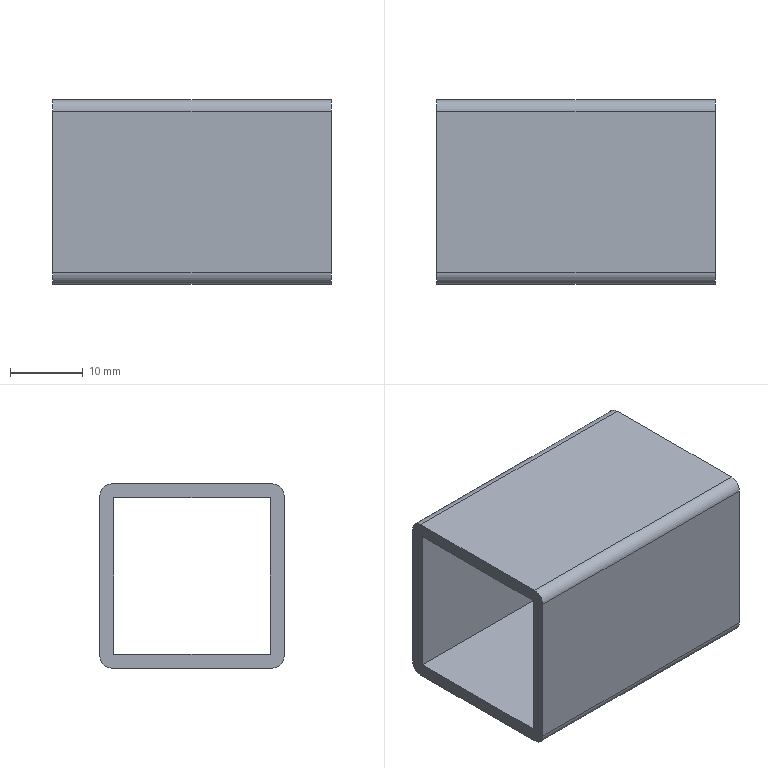Part | NX | features BREP 1 | 1 solid | 14 faces | box 38.354 x 25.4 x 25.4 mm | volume 6699 mm3 | plane 10 | cylinder 4 | commonest cylinder face diameters 3.175 x4
STEP:
#1=CARTESIAN_POINT('',(-19.177,12.7,-11.113));
#2=VERTEX_POINT('',#1);
#3=CARTESIAN_POINT('',(-19.177,12.7,11.113));
#4=VERTEX_POINT('',#3);
#5=CARTESIAN_POINT('',(-19.177,12.7,-11.113));
#6=DIRECTION('',(0.,0.,1.));
#7=VECTOR('',#6,1000.);
#8=LINE('',#5,#7);
#9=EDGE_CURVE('',#2,#4,#8,.T.);
#10=ORIENTED_EDGE('',*,*,#9,.F.);
#11=CARTESIAN_POINT('',(-19.177,11.113,-12.7));
#12=VERTEX_POINT('',#11);
#13=CARTESIAN_POINT('',(-19.177,11.113,-11.113));
#14=DIRECTION('',(-1.,0.,0.));
#15=DIRECTION('',(0.,1.,0.));
#16=AXIS2_PLACEMENT_3D('',#13,#14,#15);
#17=CIRCLE('',#16,1.587);
#18=EDGE_CURVE('',#2,#12,#17,.T.);
#19=ORIENTED_EDGE('',*,*,#18,.T.);
#20=CARTESIAN_POINT('',(-19.177,-11.113,-12.7));
#21=VERTEX_POINT('',#20);
#22=CARTESIAN_POINT('',(-19.177,-11.113,-12.7));
#23=DIRECTION('',(0.,1.,0.));
#24=VECTOR('',#23,1000.);
#25=LINE('',#22,#24);
#26=EDGE_CURVE('',#21,#12,#25,.T.);
#27=ORIENTED_EDGE('',*,*,#26,.F.);
#28=CARTESIAN_POINT('',(-19.177,-12.7,-11.113));
#29=VERTEX_POINT('',#28);
#30=CARTESIAN_POINT('',(-19.177,-11.113,-11.113));
#31=DIRECTION('',(-1.,0.,0.));
#32=DIRECTION('',(0.,0.,-1.));
#33=AXIS2_PLACEMENT_3D('',#30,#31,#32);
#34=CIRCLE('',#33,1.587);
#35=EDGE_CURVE('',#21,#29,#34,.T.);
#36=ORIENTED_EDGE('',*,*,#35,.T.);
#37=CARTESIAN_POINT('',(-19.177,-12.7,11.113));
#38=VERTEX_POINT('',#37);
#39=CARTESIAN_POINT('',(-19.177,-12.7,11.113));
#40=DIRECTION('',(0.,0.,-1.));
#41=VECTOR('',#40,1000.);
#42=LINE('',#39,#41);
#43=EDGE_CURVE('',#38,#29,#42,.T.);
#44=ORIENTED_EDGE('',*,*,#43,.F.);
#45=CARTESIAN_POINT('',(-19.177,-11.113,12.7));
#46=VERTEX_POINT('',#45);
#47=CARTESIAN_POINT('',(-19.177,-11.113,11.113));
#48=DIRECTION('',(-1.,0.,0.));
#49=DIRECTION('',(0.,-1.,0.));
#50=AXIS2_PLACEMENT_3D('',#47,#48,#49);
#51=CIRCLE('',#50,1.587);
#52=EDGE_CURVE('',#38,#46,#51,.T.);
#53=ORIENTED_EDGE('',*,*,#52,.T.);
#54=CARTESIAN_POINT('',(-19.177,11.113,12.7));
#55=VERTEX_POINT('',#54);
#56=CARTESIAN_POINT('',(-19.177,11.113,12.7));
#57=DIRECTION('',(0.,-1.,0.));
#58=VECTOR('',#57,1000.);
#59=LINE('',#56,#58);
#60=EDGE_CURVE('',#55,#46,#59,.T.);
#61=ORIENTED_EDGE('',*,*,#60,.F.);
#62=CARTESIAN_POINT('',(-19.177,11.113,11.113));
#63=DIRECTION('',(-1.,0.,0.));
#64=DIRECTION('',(0.,0.,1.));
#65=AXIS2_PLACEMENT_3D('',#62,#63,#64);
#66=CIRCLE('',#65,1.587);
#67=EDGE_CURVE('',#55,#4,#66,.T.);
#68=ORIENTED_EDGE('',*,*,#67,.T.);
#69=EDGE_LOOP('',(#10,#19,#27,#36,#44,#53,#61,#68));
#70=FACE_BOUND('',#69,.T.);
#71=CARTESIAN_POINT('',(-19.177,10.82,10.82));
#72=VERTEX_POINT('',#71);
#73=CARTESIAN_POINT('',(-19.177,10.82,-10.82));
#74=VERTEX_POINT('',#73);
#75=CARTESIAN_POINT('',(-19.177,10.82,10.82));
#76=DIRECTION('',(0.,0.,-1.));
#77=VECTOR('',#76,1000.);
#78=LINE('',#75,#77);
#79=EDGE_CURVE('',#72,#74,#78,.T.);
#80=ORIENTED_EDGE('',*,*,#79,.F.);
#81=CARTESIAN_POINT('',(-19.177,-10.82,10.82));
#82=VERTEX_POINT('',#81);
#83=CARTESIAN_POINT('',(-19.177,-10.82,10.82));
#84=DIRECTION('',(0.,1.,0.));
#85=VECTOR('',#84,1000.);
#86=LINE('',#83,#85);
#87=EDGE_CURVE('',#82,#72,#86,.T.);
#88=ORIENTED_EDGE('',*,*,#87,.F.);
#89=CARTESIAN_POINT('',(-19.177,-10.82,-10.82));
#90=VERTEX_POINT('',#89);
#91=CARTESIAN_POINT('',(-19.177,-10.82,-10.82));
#92=DIRECTION('',(0.,0.,1.));
#93=VECTOR('',#92,1000.);
#94=LINE('',#91,#93);
#95=EDGE_CURVE('',#90,#82,#94,.T.);
#96=ORIENTED_EDGE('',*,*,#95,.F.);
#97=CARTESIAN_POINT('',(-19.177,10.82,-10.82));
#98=DIRECTION('',(0.,-1.,0.));
#99=VECTOR('',#98,1000.);
#100=LINE('',#97,#99);
#101=EDGE_CURVE('',#74,#90,#100,.T.);
#102=ORIENTED_EDGE('',*,*,#101,.F.);
#103=EDGE_LOOP('',(#80,#88,#96,#102));
#104=FACE_BOUND('',#103,.T.);
#105=CARTESIAN_POINT('',(-19.177,0.,0.));
#106=DIRECTION('',(1.,0.,0.));
#107=DIRECTION('',(0.,1.,0.));
#108=AXIS2_PLACEMENT_3D('',#105,#106,#107);
#109=PLANE('',#108);
#110=ADVANCED_FACE('',(#70,#104),#109,.F.);
#111=CARTESIAN_POINT('',(19.177,-10.82,-10.82));
#112=VERTEX_POINT('',#111);
#113=CARTESIAN_POINT('',(-19.177,-10.82,-10.82));
#114=DIRECTION('',(1.,0.,0.));
#115=VECTOR('',#114,1000.);
#116=LINE('',#113,#115);
#117=EDGE_CURVE('',#90,#112,#116,.T.);
#118=ORIENTED_EDGE('',*,*,#117,.T.);
#119=CARTESIAN_POINT('',(19.177,10.82,-10.82));
#120=VERTEX_POINT('',#119);
#121=CARTESIAN_POINT('',(19.177,10.82,-10.82));
#122=DIRECTION('',(0.,-1.,0.));
#123=VECTOR('',#122,1000.);
#124=LINE('',#121,#123);
#125=EDGE_CURVE('',#120,#112,#124,.T.);
#126=ORIENTED_EDGE('',*,*,#125,.F.);
#127=CARTESIAN_POINT('',(-19.177,10.82,-10.82));
#128=DIRECTION('',(1.,0.,0.));
#129=VECTOR('',#128,1000.);
#130=LINE('',#127,#129);
#131=EDGE_CURVE('',#74,#120,#130,.T.);
#132=ORIENTED_EDGE('',*,*,#131,.F.);
#133=ORIENTED_EDGE('',*,*,#101,.T.);
#134=EDGE_LOOP('',(#118,#126,#132,#133));
#135=FACE_BOUND('',#134,.T.);
#136=CARTESIAN_POINT('',(-19.177,10.82,-10.82));
#137=DIRECTION('',(0.,0.,1.));
#138=DIRECTION('',(1.,0.,0.));
#139=AXIS2_PLACEMENT_3D('',#136,#137,#138);
#140=PLANE('',#139);
#141=ADVANCED_FACE('',(#135),#140,.T.);
#142=ORIENTED_EDGE('',*,*,#131,.T.);
#143=CARTESIAN_POINT('',(19.177,10.82,10.82));
#144=VERTEX_POINT('',#143);
#145=CARTESIAN_POINT('',(19.177,10.82,10.82));
#146=DIRECTION('',(0.,0.,-1.));
#147=VECTOR('',#146,1000.);
#148=LINE('',#145,#147);
#149=EDGE_CURVE('',#144,#120,#148,.T.);
#150=ORIENTED_EDGE('',*,*,#149,.F.);
#151=CARTESIAN_POINT('',(-19.177,10.82,10.82));
#152=DIRECTION('',(1.,0.,0.));
#153=VECTOR('',#152,1000.);
#154=LINE('',#151,#153);
#155=EDGE_CURVE('',#72,#144,#154,.T.);
#156=ORIENTED_EDGE('',*,*,#155,.F.);
#157=ORIENTED_EDGE('',*,*,#79,.T.);
#158=EDGE_LOOP('',(#142,#150,#156,#157));
#159=FACE_BOUND('',#158,.T.);
#160=CARTESIAN_POINT('',(-19.177,10.82,10.82));
#161=DIRECTION('',(0.,-1.,0.));
#162=DIRECTION('',(0.,0.,-1.));
#163=AXIS2_PLACEMENT_3D('',#160,#161,#162);
#164=PLANE('',#163);
#165=ADVANCED_FACE('',(#159),#164,.T.);
#166=ORIENTED_EDGE('',*,*,#155,.T.);
#167=CARTESIAN_POINT('',(19.177,-10.82,10.82));
#168=VERTEX_POINT('',#167);
#169=CARTESIAN_POINT('',(19.177,-10.82,10.82));
#170=DIRECTION('',(0.,1.,0.));
#171=VECTOR('',#170,1000.);
#172=LINE('',#169,#171);
#173=EDGE_CURVE('',#168,#144,#172,.T.);
#174=ORIENTED_EDGE('',*,*,#173,.F.);
#175=CARTESIAN_POINT('',(-19.177,-10.82,10.82));
#176=DIRECTION('',(1.,0.,0.));
#177=VECTOR('',#176,1000.);
#178=LINE('',#175,#177);
#179=EDGE_CURVE('',#82,#168,#178,.T.);
#180=ORIENTED_EDGE('',*,*,#179,.F.);
#181=ORIENTED_EDGE('',*,*,#87,.T.);
#182=EDGE_LOOP('',(#166,#174,#180,#181));
#183=FACE_BOUND('',#182,.T.);
#184=CARTESIAN_POINT('',(-19.177,-10.82,10.82));
#185=DIRECTION('',(0.,0.,-1.));
#186=DIRECTION('',(0.,-1.,0.));
#187=AXIS2_PLACEMENT_3D('',#184,#185,#186);
#188=PLANE('',#187);
#189=ADVANCED_FACE('',(#183),#188,.T.);
#190=ORIENTED_EDGE('',*,*,#179,.T.);
#191=CARTESIAN_POINT('',(19.177,-10.82,-10.82));
#192=DIRECTION('',(0.,0.,1.));
#193=VECTOR('',#192,1000.);
#194=LINE('',#191,#193);
#195=EDGE_CURVE('',#112,#168,#194,.T.);
#196=ORIENTED_EDGE('',*,*,#195,.F.);
#197=ORIENTED_EDGE('',*,*,#117,.F.);
#198=ORIENTED_EDGE('',*,*,#95,.T.);
#199=EDGE_LOOP('',(#190,#196,#197,#198));
#200=FACE_BOUND('',#199,.T.);
#201=CARTESIAN_POINT('',(-19.177,-10.82,-10.82));
#202=DIRECTION('',(0.,1.,0.));
#203=DIRECTION('',(1.,0.,0.));
#204=AXIS2_PLACEMENT_3D('',#201,#202,#203);
#205=PLANE('',#204);
#206=ADVANCED_FACE('',(#200),#205,.T.);
#207=CARTESIAN_POINT('',(19.177,11.113,12.7));
#208=VERTEX_POINT('',#207);
#209=CARTESIAN_POINT('',(19.177,-11.113,12.7));
#210=VERTEX_POINT('',#209);
#211=CARTESIAN_POINT('',(19.177,11.113,12.7));
#212=DIRECTION('',(0.,-1.,0.));
#213=VECTOR('',#212,1000.);
#214=LINE('',#211,#213);
#215=EDGE_CURVE('',#208,#210,#214,.T.);
#216=ORIENTED_EDGE('',*,*,#215,.T.);
#217=CARTESIAN_POINT('',(19.177,-12.7,11.113));
#218=VERTEX_POINT('',#217);
#219=CARTESIAN_POINT('',(19.177,-11.113,11.113));
#220=DIRECTION('',(1.,0.,0.));
#221=DIRECTION('',(0.,0.,1.));
#222=AXIS2_PLACEMENT_3D('',#219,#220,#221);
#223=CIRCLE('',#222,1.587);
#224=EDGE_CURVE('',#210,#218,#223,.T.);
#225=ORIENTED_EDGE('',*,*,#224,.T.);
#226=CARTESIAN_POINT('',(19.177,-12.7,-11.113));
#227=VERTEX_POINT('',#226);
#228=CARTESIAN_POINT('',(19.177,-12.7,11.113));
#229=DIRECTION('',(0.,0.,-1.));
#230=VECTOR('',#229,1000.);
#231=LINE('',#228,#230);
#232=EDGE_CURVE('',#218,#227,#231,.T.);
#233=ORIENTED_EDGE('',*,*,#232,.T.);
#234=CARTESIAN_POINT('',(19.177,-11.113,-12.7));
#235=VERTEX_POINT('',#234);
#236=CARTESIAN_POINT('',(19.177,-11.113,-11.113));
#237=DIRECTION('',(1.,0.,0.));
#238=DIRECTION('',(0.,-1.,0.));
#239=AXIS2_PLACEMENT_3D('',#236,#237,#238);
#240=CIRCLE('',#239,1.587);
#241=EDGE_CURVE('',#227,#235,#240,.T.);
#242=ORIENTED_EDGE('',*,*,#241,.T.);
#243=CARTESIAN_POINT('',(19.177,11.113,-12.7));
#244=VERTEX_POINT('',#243);
#245=CARTESIAN_POINT('',(19.177,-11.113,-12.7));
#246=DIRECTION('',(0.,1.,0.));
#247=VECTOR('',#246,1000.);
#248=LINE('',#245,#247);
#249=EDGE_CURVE('',#235,#244,#248,.T.);
#250=ORIENTED_EDGE('',*,*,#249,.T.);
#251=CARTESIAN_POINT('',(19.177,12.7,-11.113));
#252=VERTEX_POINT('',#251);
#253=CARTESIAN_POINT('',(19.177,11.113,-11.113));
#254=DIRECTION('',(1.,0.,0.));
#255=DIRECTION('',(0.,0.,-1.));
#256=AXIS2_PLACEMENT_3D('',#253,#254,#255);
#257=CIRCLE('',#256,1.587);
#258=EDGE_CURVE('',#244,#252,#257,.T.);
#259=ORIENTED_EDGE('',*,*,#258,.T.);
#260=CARTESIAN_POINT('',(19.177,12.7,11.113));
#261=VERTEX_POINT('',#260);
#262=CARTESIAN_POINT('',(19.177,12.7,-11.113));
#263=DIRECTION('',(0.,0.,1.));
#264=VECTOR('',#263,1000.);
#265=LINE('',#262,#264);
#266=EDGE_CURVE('',#252,#261,#265,.T.);
#267=ORIENTED_EDGE('',*,*,#266,.T.);
#268=CARTESIAN_POINT('',(19.177,11.113,11.113));
#269=DIRECTION('',(1.,0.,0.));
#270=DIRECTION('',(0.,1.,0.));
#271=AXIS2_PLACEMENT_3D('',#268,#269,#270);
#272=CIRCLE('',#271,1.587);
#273=EDGE_CURVE('',#261,#208,#272,.T.);
#274=ORIENTED_EDGE('',*,*,#273,.T.);
#275=EDGE_LOOP('',(#216,#225,#233,#242,#250,#259,#267,#274));
#276=FACE_BOUND('',#275,.T.);
#277=ORIENTED_EDGE('',*,*,#195,.T.);
#278=ORIENTED_EDGE('',*,*,#173,.T.);
#279=ORIENTED_EDGE('',*,*,#149,.T.);
#280=ORIENTED_EDGE('',*,*,#125,.T.);
#281=EDGE_LOOP('',(#277,#278,#279,#280));
#282=FACE_BOUND('',#281,.T.);
#283=CARTESIAN_POINT('',(19.177,0.,0.));
#284=DIRECTION('',(1.,0.,0.));
#285=DIRECTION('',(0.,1.,0.));
#286=AXIS2_PLACEMENT_3D('',#283,#284,#285);
#287=PLANE('',#286);
#288=ADVANCED_FACE('',(#276,#282),#287,.T.);
#289=ORIENTED_EDGE('',*,*,#273,.F.);
#290=CARTESIAN_POINT('',(19.177,12.7,11.113));
#291=DIRECTION('',(-1.,0.,0.));
#292=VECTOR('',#291,1000.);
#293=LINE('',#290,#292);
#294=EDGE_CURVE('',#261,#4,#293,.T.);
#295=ORIENTED_EDGE('',*,*,#294,.T.);
#296=ORIENTED_EDGE('',*,*,#67,.F.);
#297=CARTESIAN_POINT('',(19.177,11.113,12.7));
#298=DIRECTION('',(-1.,0.,0.));
#299=VECTOR('',#298,1000.);
#300=LINE('',#297,#299);
#301=EDGE_CURVE('',#208,#55,#300,.T.);
#302=ORIENTED_EDGE('',*,*,#301,.F.);
#303=EDGE_LOOP('',(#289,#295,#296,#302));
#304=FACE_BOUND('',#303,.T.);
#305=CARTESIAN_POINT('',(19.259,11.113,11.113));
#306=DIRECTION('',(-1.,0.,0.));
#307=DIRECTION('',(0.,0.,1.));
#308=AXIS2_PLACEMENT_3D('',#305,#306,#307);
#309=CYLINDRICAL_SURFACE('',#308,1.587);
#310=ADVANCED_FACE('',(#304),#309,.T.);
#311=ORIENTED_EDGE('',*,*,#60,.T.);
#312=CARTESIAN_POINT('',(19.177,-11.113,12.7));
#313=DIRECTION('',(-1.,0.,0.));
#314=VECTOR('',#313,1000.);
#315=LINE('',#312,#314);
#316=EDGE_CURVE('',#210,#46,#315,.T.);
#317=ORIENTED_EDGE('',*,*,#316,.F.);
#318=ORIENTED_EDGE('',*,*,#215,.F.);
#319=ORIENTED_EDGE('',*,*,#301,.T.);
#320=EDGE_LOOP('',(#311,#317,#318,#319));
#321=FACE_BOUND('',#320,.T.);
#322=CARTESIAN_POINT('',(-19.177,12.7,12.7));
#323=DIRECTION('',(0.,0.,1.));
#324=DIRECTION('',(1.,0.,0.));
#325=AXIS2_PLACEMENT_3D('',#322,#323,#324);
#326=PLANE('',#325);
#327=ADVANCED_FACE('',(#321),#326,.T.);
#328=ORIENTED_EDGE('',*,*,#224,.F.);
#329=ORIENTED_EDGE('',*,*,#316,.T.);
#330=ORIENTED_EDGE('',*,*,#52,.F.);
#331=CARTESIAN_POINT('',(19.177,-12.7,11.113));
#332=DIRECTION('',(-1.,0.,0.));
#333=VECTOR('',#332,1000.);
#334=LINE('',#331,#333);
#335=EDGE_CURVE('',#218,#38,#334,.T.);
#336=ORIENTED_EDGE('',*,*,#335,.F.);
#337=EDGE_LOOP('',(#328,#329,#330,#336));
#338=FACE_BOUND('',#337,.T.);
#339=CARTESIAN_POINT('',(19.259,-11.113,11.113));
#340=DIRECTION('',(-1.,0.,0.));
#341=DIRECTION('',(0.,-1.,0.));
#342=AXIS2_PLACEMENT_3D('',#339,#340,#341);
#343=CYLINDRICAL_SURFACE('',#342,1.587);
#344=ADVANCED_FACE('',(#338),#343,.T.);
#345=ORIENTED_EDGE('',*,*,#43,.T.);
#346=CARTESIAN_POINT('',(19.177,-12.7,-11.113));
#347=DIRECTION('',(-1.,0.,0.));
#348=VECTOR('',#347,1000.);
#349=LINE('',#346,#348);
#350=EDGE_CURVE('',#227,#29,#349,.T.);
#351=ORIENTED_EDGE('',*,*,#350,.F.);
#352=ORIENTED_EDGE('',*,*,#232,.F.);
#353=ORIENTED_EDGE('',*,*,#335,.T.);
#354=EDGE_LOOP('',(#345,#351,#352,#353));
#355=FACE_BOUND('',#354,.T.);
#356=CARTESIAN_POINT('',(-19.177,-12.7,12.7));
#357=DIRECTION('',(0.,-1.,0.));
#358=DIRECTION('',(0.,0.,-1.));
#359=AXIS2_PLACEMENT_3D('',#356,#357,#358);
#360=PLANE('',#359);
#361=ADVANCED_FACE('',(#355),#360,.T.);
#362=ORIENTED_EDGE('',*,*,#241,.F.);
#363=ORIENTED_EDGE('',*,*,#350,.T.);
#364=ORIENTED_EDGE('',*,*,#35,.F.);
#365=CARTESIAN_POINT('',(19.177,-11.113,-12.7));
#366=DIRECTION('',(-1.,0.,0.));
#367=VECTOR('',#366,1000.);
#368=LINE('',#365,#367);
#369=EDGE_CURVE('',#235,#21,#368,.T.);
#370=ORIENTED_EDGE('',*,*,#369,.F.);
#371=EDGE_LOOP('',(#362,#363,#364,#370));
#372=FACE_BOUND('',#371,.T.);
#373=CARTESIAN_POINT('',(19.259,-11.113,-11.113));
#374=DIRECTION('',(-1.,0.,0.));
#375=DIRECTION('',(0.,0.,-1.));
#376=AXIS2_PLACEMENT_3D('',#373,#374,#375);
#377=CYLINDRICAL_SURFACE('',#376,1.587);
#378=ADVANCED_FACE('',(#372),#377,.T.);
#379=ORIENTED_EDGE('',*,*,#249,.F.);
#380=ORIENTED_EDGE('',*,*,#369,.T.);
#381=ORIENTED_EDGE('',*,*,#26,.T.);
#382=CARTESIAN_POINT('',(19.177,11.113,-12.7));
#383=DIRECTION('',(-1.,0.,0.));
#384=VECTOR('',#383,1000.);
#385=LINE('',#382,#384);
#386=EDGE_CURVE('',#244,#12,#385,.T.);
#387=ORIENTED_EDGE('',*,*,#386,.F.);
#388=EDGE_LOOP('',(#379,#380,#381,#387));
#389=FACE_BOUND('',#388,.T.);
#390=CARTESIAN_POINT('',(-19.177,-12.7,-12.7));
#391=DIRECTION('',(0.,0.,-1.));
#392=DIRECTION('',(0.,-1.,0.));
#393=AXIS2_PLACEMENT_3D('',#390,#391,#392);
#394=PLANE('',#393);
#395=ADVANCED_FACE('',(#389),#394,.T.);
#396=ORIENTED_EDGE('',*,*,#258,.F.);
#397=ORIENTED_EDGE('',*,*,#386,.T.);
#398=ORIENTED_EDGE('',*,*,#18,.F.);
#399=CARTESIAN_POINT('',(19.177,12.7,-11.113));
#400=DIRECTION('',(-1.,0.,0.));
#401=VECTOR('',#400,1000.);
#402=LINE('',#399,#401);
#403=EDGE_CURVE('',#252,#2,#402,.T.);
#404=ORIENTED_EDGE('',*,*,#403,.F.);
#405=EDGE_LOOP('',(#396,#397,#398,#404));
#406=FACE_BOUND('',#405,.T.);
#407=CARTESIAN_POINT('',(19.259,11.113,-11.113));
#408=DIRECTION('',(-1.,0.,0.));
#409=DIRECTION('',(0.,1.,0.));
#410=AXIS2_PLACEMENT_3D('',#407,#408,#409);
#411=CYLINDRICAL_SURFACE('',#410,1.587);
#412=ADVANCED_FACE('',(#406),#411,.T.);
#413=ORIENTED_EDGE('',*,*,#266,.F.);
#414=ORIENTED_EDGE('',*,*,#403,.T.);
#415=ORIENTED_EDGE('',*,*,#9,.T.);
#416=ORIENTED_EDGE('',*,*,#294,.F.);
#417=EDGE_LOOP('',(#413,#414,#415,#416));
#418=FACE_BOUND('',#417,.T.);
#419=CARTESIAN_POINT('',(-19.177,12.7,-12.7));
#420=DIRECTION('',(0.,1.,0.));
#421=DIRECTION('',(1.,0.,0.));
#422=AXIS2_PLACEMENT_3D('',#419,#420,#421);
#423=PLANE('',#422);
#424=ADVANCED_FACE('',(#418),#423,.T.);
#425=CLOSED_SHELL('',(#110,#141,#165,#189,#206,#288,#310,#327,#344,#361,#378,#395,#412,#424));
#426=MANIFOLD_SOLID_BREP('',#425);
#427=(LENGTH_UNIT()NAMED_UNIT(*)SI_UNIT(.MILLI.,.METRE.));
#428=UNCERTAINTY_MEASURE_WITH_UNIT(LENGTH_MEASURE(0.00001),#427,'','');
#429=(NAMED_UNIT(*)PLANE_ANGLE_UNIT()SI_UNIT($,.RADIAN.));
#430=(NAMED_UNIT(*)SI_UNIT($,.STERADIAN.)SOLID_ANGLE_UNIT());
#431=(GEOMETRIC_REPRESENTATION_CONTEXT(3)GLOBAL_UNCERTAINTY_ASSIGNED_CONTEXT((#428))GLOBAL_UNIT_ASSIGNED_CONTEXT((#427,#429,#430))REPRESENTATION_CONTEXT('',''));
#432=ADVANCED_BREP_SHAPE_REPRESENTATION('',(#426),#431);